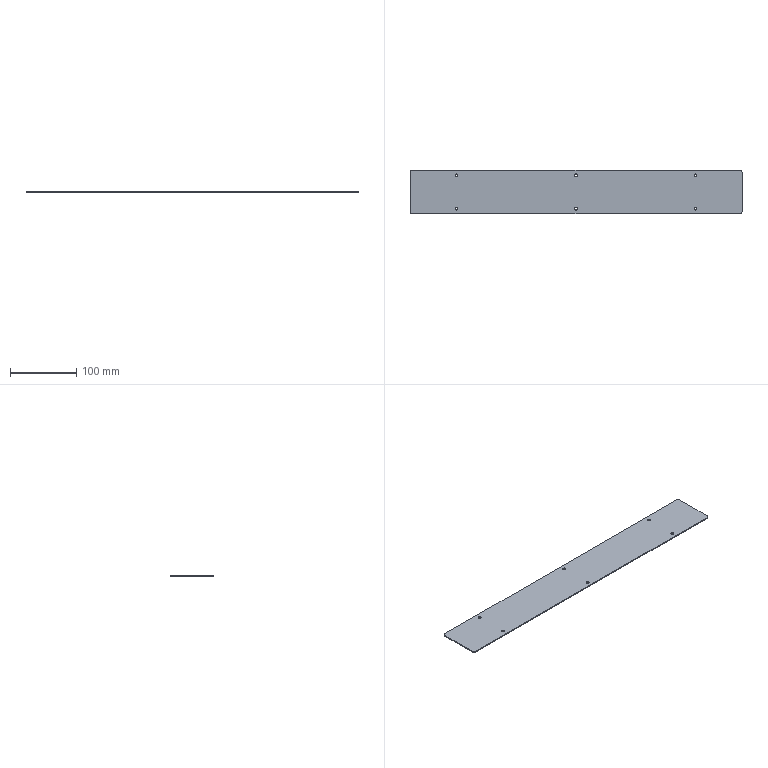Part | SolidWorks | features Fillet 1, FlatPattern 1, ICE 1, LPattern 1, SMBaseFlange 1, SheetMetal 1 | 1 solid | 22 faces | box 500 x 65 x 1.5 mm | volume 48608 mm3 | cylinder 16 | plane 6 | commonest cylinder face diameters 4.3 x12 6 x4
STEP:
#1=CARTESIAN_POINT('',(2.15,25.,-1.5));
#2=VERTEX_POINT('',#1);
#3=CARTESIAN_POINT('',(-2.15,25.,-1.5));
#4=VERTEX_POINT('',#3);
#5=CARTESIAN_POINT('',(0.,25.,-1.5));
#6=DIRECTION('',(0.,0.,-1.));
#7=DIRECTION('',(-1.,0.,0.));
#8=AXIS2_PLACEMENT_3D('',#5,#6,#7);
#9=CIRCLE('',#8,2.15);
#10=EDGE_CURVE('',#2,#4,#9,.T.);
#11=ORIENTED_EDGE('',*,*,#10,.T.);
#12=CARTESIAN_POINT('',(-2.15,25.,0.));
#13=VERTEX_POINT('',#12);
#14=CARTESIAN_POINT('',(-2.15,25.,-10.));
#15=DIRECTION('',(0.,0.,1.));
#16=VECTOR('',#15,1000.);
#17=LINE('',#14,#16);
#18=EDGE_CURVE('',#4,#13,#17,.T.);
#19=ORIENTED_EDGE('',*,*,#18,.T.);
#20=CARTESIAN_POINT('',(2.15,25.,0.));
#21=VERTEX_POINT('',#20);
#22=CARTESIAN_POINT('',(0.,25.,0.));
#23=DIRECTION('',(0.,0.,1.));
#24=DIRECTION('',(1.,0.,0.));
#25=AXIS2_PLACEMENT_3D('',#22,#23,#24);
#26=CIRCLE('',#25,2.15);
#27=EDGE_CURVE('',#13,#21,#26,.T.);
#28=ORIENTED_EDGE('',*,*,#27,.T.);
#29=CARTESIAN_POINT('',(2.15,25.,-10.));
#30=DIRECTION('',(0.,0.,1.));
#31=VECTOR('',#30,1000.);
#32=LINE('',#29,#31);
#33=EDGE_CURVE('',#2,#21,#32,.T.);
#34=ORIENTED_EDGE('',*,*,#33,.F.);
#35=EDGE_LOOP('',(#11,#19,#28,#34));
#36=FACE_OUTER_BOUND('',#35,.T.);
#37=CARTESIAN_POINT('',(0.,25.,-10.));
#38=DIRECTION('',(0.,0.,1.));
#39=DIRECTION('',(1.,0.,0.));
#40=AXIS2_PLACEMENT_3D('',#37,#38,#39);
#41=CYLINDRICAL_SURFACE('',#40,2.15);
#42=ADVANCED_FACE('',(#36),#41,.F.);
#43=CARTESIAN_POINT('',(-177.85,25.,-1.5));
#44=VERTEX_POINT('',#43);
#45=CARTESIAN_POINT('',(-182.15,25.,-1.5));
#46=VERTEX_POINT('',#45);
#47=CARTESIAN_POINT('',(-180.,25.,-1.5));
#48=DIRECTION('',(0.,0.,-1.));
#49=DIRECTION('',(-1.,0.,0.));
#50=AXIS2_PLACEMENT_3D('',#47,#48,#49);
#51=CIRCLE('',#50,2.15);
#52=EDGE_CURVE('',#44,#46,#51,.T.);
#53=ORIENTED_EDGE('',*,*,#52,.T.);
#54=CARTESIAN_POINT('',(-182.15,25.,0.));
#55=VERTEX_POINT('',#54);
#56=CARTESIAN_POINT('',(-182.15,25.,-10.));
#57=DIRECTION('',(0.,0.,1.));
#58=VECTOR('',#57,1000.);
#59=LINE('',#56,#58);
#60=EDGE_CURVE('',#46,#55,#59,.T.);
#61=ORIENTED_EDGE('',*,*,#60,.T.);
#62=CARTESIAN_POINT('',(-177.85,25.,0.));
#63=VERTEX_POINT('',#62);
#64=CARTESIAN_POINT('',(-180.,25.,0.));
#65=DIRECTION('',(0.,0.,1.));
#66=DIRECTION('',(1.,0.,0.));
#67=AXIS2_PLACEMENT_3D('',#64,#65,#66);
#68=CIRCLE('',#67,2.15);
#69=EDGE_CURVE('',#55,#63,#68,.T.);
#70=ORIENTED_EDGE('',*,*,#69,.T.);
#71=CARTESIAN_POINT('',(-177.85,25.,-10.));
#72=DIRECTION('',(0.,0.,1.));
#73=VECTOR('',#72,1000.);
#74=LINE('',#71,#73);
#75=EDGE_CURVE('',#44,#63,#74,.T.);
#76=ORIENTED_EDGE('',*,*,#75,.F.);
#77=EDGE_LOOP('',(#53,#61,#70,#76));
#78=FACE_OUTER_BOUND('',#77,.T.);
#79=CARTESIAN_POINT('',(-180.,25.,-10.));
#80=DIRECTION('',(0.,0.,1.));
#81=DIRECTION('',(1.,0.,0.));
#82=AXIS2_PLACEMENT_3D('',#79,#80,#81);
#83=CYLINDRICAL_SURFACE('',#82,2.15);
#84=ADVANCED_FACE('',(#78),#83,.F.);
#85=CARTESIAN_POINT('',(182.15,25.,-1.5));
#86=VERTEX_POINT('',#85);
#87=CARTESIAN_POINT('',(177.85,25.,-1.5));
#88=VERTEX_POINT('',#87);
#89=CARTESIAN_POINT('',(180.,25.,-1.5));
#90=DIRECTION('',(0.,0.,-1.));
#91=DIRECTION('',(-1.,0.,0.));
#92=AXIS2_PLACEMENT_3D('',#89,#90,#91);
#93=CIRCLE('',#92,2.15);
#94=EDGE_CURVE('',#86,#88,#93,.T.);
#95=ORIENTED_EDGE('',*,*,#94,.T.);
#96=CARTESIAN_POINT('',(177.85,25.,0.));
#97=VERTEX_POINT('',#96);
#98=CARTESIAN_POINT('',(177.85,25.,-10.));
#99=DIRECTION('',(0.,0.,1.));
#100=VECTOR('',#99,1000.);
#101=LINE('',#98,#100);
#102=EDGE_CURVE('',#88,#97,#101,.T.);
#103=ORIENTED_EDGE('',*,*,#102,.T.);
#104=CARTESIAN_POINT('',(182.15,25.,0.));
#105=VERTEX_POINT('',#104);
#106=CARTESIAN_POINT('',(180.,25.,0.));
#107=DIRECTION('',(0.,0.,1.));
#108=DIRECTION('',(1.,0.,0.));
#109=AXIS2_PLACEMENT_3D('',#106,#107,#108);
#110=CIRCLE('',#109,2.15);
#111=EDGE_CURVE('',#97,#105,#110,.T.);
#112=ORIENTED_EDGE('',*,*,#111,.T.);
#113=CARTESIAN_POINT('',(182.15,25.,-10.));
#114=DIRECTION('',(0.,0.,1.));
#115=VECTOR('',#114,1000.);
#116=LINE('',#113,#115);
#117=EDGE_CURVE('',#86,#105,#116,.T.);
#118=ORIENTED_EDGE('',*,*,#117,.F.);
#119=EDGE_LOOP('',(#95,#103,#112,#118));
#120=FACE_OUTER_BOUND('',#119,.T.);
#121=CARTESIAN_POINT('',(180.,25.,-10.));
#122=DIRECTION('',(0.,0.,1.));
#123=DIRECTION('',(1.,0.,0.));
#124=AXIS2_PLACEMENT_3D('',#121,#122,#123);
#125=CYLINDRICAL_SURFACE('',#124,2.15);
#126=ADVANCED_FACE('',(#120),#125,.F.);
#127=CARTESIAN_POINT('',(-177.85,-25.,-1.5));
#128=VERTEX_POINT('',#127);
#129=CARTESIAN_POINT('',(-182.15,-25.,-1.5));
#130=VERTEX_POINT('',#129);
#131=CARTESIAN_POINT('',(-180.,-25.,-1.5));
#132=DIRECTION('',(0.,0.,-1.));
#133=DIRECTION('',(-1.,0.,0.));
#134=AXIS2_PLACEMENT_3D('',#131,#132,#133);
#135=CIRCLE('',#134,2.15);
#136=EDGE_CURVE('',#128,#130,#135,.T.);
#137=ORIENTED_EDGE('',*,*,#136,.T.);
#138=CARTESIAN_POINT('',(-182.15,-25.,0.));
#139=VERTEX_POINT('',#138);
#140=CARTESIAN_POINT('',(-182.15,-25.,-10.));
#141=DIRECTION('',(0.,0.,1.));
#142=VECTOR('',#141,1000.);
#143=LINE('',#140,#142);
#144=EDGE_CURVE('',#130,#139,#143,.T.);
#145=ORIENTED_EDGE('',*,*,#144,.T.);
#146=CARTESIAN_POINT('',(-177.85,-25.,0.));
#147=VERTEX_POINT('',#146);
#148=CARTESIAN_POINT('',(-180.,-25.,0.));
#149=DIRECTION('',(0.,0.,1.));
#150=DIRECTION('',(1.,0.,0.));
#151=AXIS2_PLACEMENT_3D('',#148,#149,#150);
#152=CIRCLE('',#151,2.15);
#153=EDGE_CURVE('',#139,#147,#152,.T.);
#154=ORIENTED_EDGE('',*,*,#153,.T.);
#155=CARTESIAN_POINT('',(-177.85,-25.,-10.));
#156=DIRECTION('',(0.,0.,1.));
#157=VECTOR('',#156,1000.);
#158=LINE('',#155,#157);
#159=EDGE_CURVE('',#128,#147,#158,.T.);
#160=ORIENTED_EDGE('',*,*,#159,.F.);
#161=EDGE_LOOP('',(#137,#145,#154,#160));
#162=FACE_OUTER_BOUND('',#161,.T.);
#163=CARTESIAN_POINT('',(-180.,-25.,-10.));
#164=DIRECTION('',(0.,0.,1.));
#165=DIRECTION('',(1.,0.,0.));
#166=AXIS2_PLACEMENT_3D('',#163,#164,#165);
#167=CYLINDRICAL_SURFACE('',#166,2.15);
#168=ADVANCED_FACE('',(#162),#167,.F.);
#169=CARTESIAN_POINT('',(2.15,-25.,-1.5));
#170=VERTEX_POINT('',#169);
#171=CARTESIAN_POINT('',(-2.15,-25.,-1.5));
#172=VERTEX_POINT('',#171);
#173=CARTESIAN_POINT('',(0.,-25.,-1.5));
#174=DIRECTION('',(0.,0.,-1.));
#175=DIRECTION('',(-1.,0.,0.));
#176=AXIS2_PLACEMENT_3D('',#173,#174,#175);
#177=CIRCLE('',#176,2.15);
#178=EDGE_CURVE('',#170,#172,#177,.T.);
#179=ORIENTED_EDGE('',*,*,#178,.T.);
#180=CARTESIAN_POINT('',(-2.15,-25.,0.));
#181=VERTEX_POINT('',#180);
#182=CARTESIAN_POINT('',(-2.15,-25.,-10.));
#183=DIRECTION('',(0.,0.,1.));
#184=VECTOR('',#183,1000.);
#185=LINE('',#182,#184);
#186=EDGE_CURVE('',#172,#181,#185,.T.);
#187=ORIENTED_EDGE('',*,*,#186,.T.);
#188=CARTESIAN_POINT('',(2.15,-25.,0.));
#189=VERTEX_POINT('',#188);
#190=CARTESIAN_POINT('',(0.,-25.,0.));
#191=DIRECTION('',(0.,0.,1.));
#192=DIRECTION('',(1.,0.,0.));
#193=AXIS2_PLACEMENT_3D('',#190,#191,#192);
#194=CIRCLE('',#193,2.15);
#195=EDGE_CURVE('',#181,#189,#194,.T.);
#196=ORIENTED_EDGE('',*,*,#195,.T.);
#197=CARTESIAN_POINT('',(2.15,-25.,-10.));
#198=DIRECTION('',(0.,0.,1.));
#199=VECTOR('',#198,1000.);
#200=LINE('',#197,#199);
#201=EDGE_CURVE('',#170,#189,#200,.T.);
#202=ORIENTED_EDGE('',*,*,#201,.F.);
#203=EDGE_LOOP('',(#179,#187,#196,#202));
#204=FACE_OUTER_BOUND('',#203,.T.);
#205=CARTESIAN_POINT('',(0.,-25.,-10.));
#206=DIRECTION('',(0.,0.,1.));
#207=DIRECTION('',(1.,0.,0.));
#208=AXIS2_PLACEMENT_3D('',#205,#206,#207);
#209=CYLINDRICAL_SURFACE('',#208,2.15);
#210=ADVANCED_FACE('',(#204),#209,.F.);
#211=CARTESIAN_POINT('',(182.15,-25.,-1.5));
#212=VERTEX_POINT('',#211);
#213=CARTESIAN_POINT('',(177.85,-25.,-1.5));
#214=VERTEX_POINT('',#213);
#215=CARTESIAN_POINT('',(180.,-25.,-1.5));
#216=DIRECTION('',(0.,0.,-1.));
#217=DIRECTION('',(-1.,0.,0.));
#218=AXIS2_PLACEMENT_3D('',#215,#216,#217);
#219=CIRCLE('',#218,2.15);
#220=EDGE_CURVE('',#212,#214,#219,.T.);
#221=ORIENTED_EDGE('',*,*,#220,.T.);
#222=CARTESIAN_POINT('',(177.85,-25.,0.));
#223=VERTEX_POINT('',#222);
#224=CARTESIAN_POINT('',(177.85,-25.,-10.));
#225=DIRECTION('',(0.,0.,1.));
#226=VECTOR('',#225,1000.);
#227=LINE('',#224,#226);
#228=EDGE_CURVE('',#214,#223,#227,.T.);
#229=ORIENTED_EDGE('',*,*,#228,.T.);
#230=CARTESIAN_POINT('',(182.15,-25.,0.));
#231=VERTEX_POINT('',#230);
#232=CARTESIAN_POINT('',(180.,-25.,0.));
#233=DIRECTION('',(0.,0.,1.));
#234=DIRECTION('',(1.,0.,0.));
#235=AXIS2_PLACEMENT_3D('',#232,#233,#234);
#236=CIRCLE('',#235,2.15);
#237=EDGE_CURVE('',#223,#231,#236,.T.);
#238=ORIENTED_EDGE('',*,*,#237,.T.);
#239=CARTESIAN_POINT('',(182.15,-25.,-10.));
#240=DIRECTION('',(0.,0.,1.));
#241=VECTOR('',#240,1000.);
#242=LINE('',#239,#241);
#243=EDGE_CURVE('',#212,#231,#242,.T.);
#244=ORIENTED_EDGE('',*,*,#243,.F.);
#245=EDGE_LOOP('',(#221,#229,#238,#244));
#246=FACE_OUTER_BOUND('',#245,.T.);
#247=CARTESIAN_POINT('',(180.,-25.,-10.));
#248=DIRECTION('',(0.,0.,1.));
#249=DIRECTION('',(1.,0.,0.));
#250=AXIS2_PLACEMENT_3D('',#247,#248,#249);
#251=CYLINDRICAL_SURFACE('',#250,2.15);
#252=ADVANCED_FACE('',(#246),#251,.F.);
#253=ORIENTED_EDGE('',*,*,#228,.F.);
#254=CARTESIAN_POINT('',(180.,-25.,-1.5));
#255=DIRECTION('',(0.,0.,-1.));
#256=DIRECTION('',(-1.,0.,0.));
#257=AXIS2_PLACEMENT_3D('',#254,#255,#256);
#258=CIRCLE('',#257,2.15);
#259=EDGE_CURVE('',#214,#212,#258,.T.);
#260=ORIENTED_EDGE('',*,*,#259,.T.);
#261=ORIENTED_EDGE('',*,*,#243,.T.);
#262=CARTESIAN_POINT('',(180.,-25.,0.));
#263=DIRECTION('',(0.,0.,1.));
#264=DIRECTION('',(1.,0.,0.));
#265=AXIS2_PLACEMENT_3D('',#262,#263,#264);
#266=CIRCLE('',#265,2.15);
#267=EDGE_CURVE('',#231,#223,#266,.T.);
#268=ORIENTED_EDGE('',*,*,#267,.T.);
#269=EDGE_LOOP('',(#253,#260,#261,#268));
#270=FACE_OUTER_BOUND('',#269,.T.);
#271=CARTESIAN_POINT('',(180.,-25.,-10.));
#272=DIRECTION('',(0.,0.,1.));
#273=DIRECTION('',(1.,0.,0.));
#274=AXIS2_PLACEMENT_3D('',#271,#272,#273);
#275=CYLINDRICAL_SURFACE('',#274,2.15);
#276=ADVANCED_FACE('',(#270),#275,.F.);
#277=ORIENTED_EDGE('',*,*,#186,.F.);
#278=CARTESIAN_POINT('',(0.,-25.,-1.5));
#279=DIRECTION('',(0.,0.,-1.));
#280=DIRECTION('',(-1.,0.,0.));
#281=AXIS2_PLACEMENT_3D('',#278,#279,#280);
#282=CIRCLE('',#281,2.15);
#283=EDGE_CURVE('',#172,#170,#282,.T.);
#284=ORIENTED_EDGE('',*,*,#283,.T.);
#285=ORIENTED_EDGE('',*,*,#201,.T.);
#286=CARTESIAN_POINT('',(0.,-25.,0.));
#287=DIRECTION('',(0.,0.,1.));
#288=DIRECTION('',(1.,0.,0.));
#289=AXIS2_PLACEMENT_3D('',#286,#287,#288);
#290=CIRCLE('',#289,2.15);
#291=EDGE_CURVE('',#189,#181,#290,.T.);
#292=ORIENTED_EDGE('',*,*,#291,.T.);
#293=EDGE_LOOP('',(#277,#284,#285,#292));
#294=FACE_OUTER_BOUND('',#293,.T.);
#295=CARTESIAN_POINT('',(0.,-25.,-10.));
#296=DIRECTION('',(0.,0.,1.));
#297=DIRECTION('',(1.,0.,0.));
#298=AXIS2_PLACEMENT_3D('',#295,#296,#297);
#299=CYLINDRICAL_SURFACE('',#298,2.15);
#300=ADVANCED_FACE('',(#294),#299,.F.);
#301=ORIENTED_EDGE('',*,*,#144,.F.);
#302=CARTESIAN_POINT('',(-180.,-25.,-1.5));
#303=DIRECTION('',(0.,0.,-1.));
#304=DIRECTION('',(-1.,0.,0.));
#305=AXIS2_PLACEMENT_3D('',#302,#303,#304);
#306=CIRCLE('',#305,2.15);
#307=EDGE_CURVE('',#130,#128,#306,.T.);
#308=ORIENTED_EDGE('',*,*,#307,.T.);
#309=ORIENTED_EDGE('',*,*,#159,.T.);
#310=CARTESIAN_POINT('',(-180.,-25.,0.));
#311=DIRECTION('',(0.,0.,1.));
#312=DIRECTION('',(1.,0.,0.));
#313=AXIS2_PLACEMENT_3D('',#310,#311,#312);
#314=CIRCLE('',#313,2.15);
#315=EDGE_CURVE('',#147,#139,#314,.T.);
#316=ORIENTED_EDGE('',*,*,#315,.T.);
#317=EDGE_LOOP('',(#301,#308,#309,#316));
#318=FACE_OUTER_BOUND('',#317,.T.);
#319=CARTESIAN_POINT('',(-180.,-25.,-10.));
#320=DIRECTION('',(0.,0.,1.));
#321=DIRECTION('',(1.,0.,0.));
#322=AXIS2_PLACEMENT_3D('',#319,#320,#321);
#323=CYLINDRICAL_SURFACE('',#322,2.15);
#324=ADVANCED_FACE('',(#318),#323,.F.);
#325=ORIENTED_EDGE('',*,*,#102,.F.);
#326=CARTESIAN_POINT('',(180.,25.,-1.5));
#327=DIRECTION('',(0.,0.,-1.));
#328=DIRECTION('',(-1.,0.,0.));
#329=AXIS2_PLACEMENT_3D('',#326,#327,#328);
#330=CIRCLE('',#329,2.15);
#331=EDGE_CURVE('',#88,#86,#330,.T.);
#332=ORIENTED_EDGE('',*,*,#331,.T.);
#333=ORIENTED_EDGE('',*,*,#117,.T.);
#334=CARTESIAN_POINT('',(180.,25.,0.));
#335=DIRECTION('',(0.,0.,1.));
#336=DIRECTION('',(1.,0.,0.));
#337=AXIS2_PLACEMENT_3D('',#334,#335,#336);
#338=CIRCLE('',#337,2.15);
#339=EDGE_CURVE('',#105,#97,#338,.T.);
#340=ORIENTED_EDGE('',*,*,#339,.T.);
#341=EDGE_LOOP('',(#325,#332,#333,#340));
#342=FACE_OUTER_BOUND('',#341,.T.);
#343=CARTESIAN_POINT('',(180.,25.,-10.));
#344=DIRECTION('',(0.,0.,1.));
#345=DIRECTION('',(1.,0.,0.));
#346=AXIS2_PLACEMENT_3D('',#343,#344,#345);
#347=CYLINDRICAL_SURFACE('',#346,2.15);
#348=ADVANCED_FACE('',(#342),#347,.F.);
#349=CARTESIAN_POINT('',(250.,-29.5,-1.5));
#350=VERTEX_POINT('',#349);
#351=CARTESIAN_POINT('',(250.,29.5,-1.5));
#352=VERTEX_POINT('',#351);
#353=CARTESIAN_POINT('',(250.,-32.5,-1.5));
#354=DIRECTION('',(0.,1.,0.));
#355=VECTOR('',#354,1000.);
#356=LINE('',#353,#355);
#357=EDGE_CURVE('',#350,#352,#356,.T.);
#358=ORIENTED_EDGE('',*,*,#357,.T.);
#359=CARTESIAN_POINT('',(250.,29.5,0.));
#360=VERTEX_POINT('',#359);
#361=CARTESIAN_POINT('',(250.,29.5,-1.5));
#362=DIRECTION('',(0.,0.,1.));
#363=VECTOR('',#362,1000.);
#364=LINE('',#361,#363);
#365=EDGE_CURVE('',#352,#360,#364,.T.);
#366=ORIENTED_EDGE('',*,*,#365,.T.);
#367=CARTESIAN_POINT('',(250.,-29.5,0.));
#368=VERTEX_POINT('',#367);
#369=CARTESIAN_POINT('',(250.,-32.5,0.));
#370=DIRECTION('',(0.,1.,0.));
#371=VECTOR('',#370,1000.);
#372=LINE('',#369,#371);
#373=EDGE_CURVE('',#368,#360,#372,.T.);
#374=ORIENTED_EDGE('',*,*,#373,.F.);
#375=CARTESIAN_POINT('',(250.,-29.5,-1.5));
#376=DIRECTION('',(0.,0.,-1.));
#377=VECTOR('',#376,1000.);
#378=LINE('',#375,#377);
#379=EDGE_CURVE('',#368,#350,#378,.T.);
#380=ORIENTED_EDGE('',*,*,#379,.T.);
#381=EDGE_LOOP('',(#358,#366,#374,#380));
#382=FACE_OUTER_BOUND('',#381,.T.);
#383=CARTESIAN_POINT('',(250.,-32.5,-1.5));
#384=DIRECTION('',(1.,0.,0.));
#385=DIRECTION('',(0.,0.,-1.));
#386=AXIS2_PLACEMENT_3D('',#383,#384,#385);
#387=PLANE('',#386);
#388=ADVANCED_FACE('',(#382),#387,.T.);
#389=CARTESIAN_POINT('',(-247.,-32.5,0.));
#390=VERTEX_POINT('',#389);
#391=CARTESIAN_POINT('',(247.,-32.5,0.));
#392=VERTEX_POINT('',#391);
#393=CARTESIAN_POINT('',(-250.,-32.5,0.));
#394=DIRECTION('',(1.,0.,0.));
#395=VECTOR('',#394,1000.);
#396=LINE('',#393,#395);
#397=EDGE_CURVE('',#390,#392,#396,.T.);
#398=ORIENTED_EDGE('',*,*,#397,.F.);
#399=CARTESIAN_POINT('',(-247.,-32.5,-1.5));
#400=VERTEX_POINT('',#399);
#401=CARTESIAN_POINT('',(-247.,-32.5,-1.5));
#402=DIRECTION('',(0.,0.,-1.));
#403=VECTOR('',#402,1000.);
#404=LINE('',#401,#403);
#405=EDGE_CURVE('',#390,#400,#404,.T.);
#406=ORIENTED_EDGE('',*,*,#405,.T.);
#407=CARTESIAN_POINT('',(247.,-32.5,-1.5));
#408=VERTEX_POINT('',#407);
#409=CARTESIAN_POINT('',(-250.,-32.5,-1.5));
#410=DIRECTION('',(1.,0.,0.));
#411=VECTOR('',#410,1000.);
#412=LINE('',#409,#411);
#413=EDGE_CURVE('',#400,#408,#412,.T.);
#414=ORIENTED_EDGE('',*,*,#413,.T.);
#415=CARTESIAN_POINT('',(247.,-32.5,-1.5));
#416=DIRECTION('',(0.,0.,1.));
#417=VECTOR('',#416,1000.);
#418=LINE('',#415,#417);
#419=EDGE_CURVE('',#408,#392,#418,.T.);
#420=ORIENTED_EDGE('',*,*,#419,.T.);
#421=EDGE_LOOP('',(#398,#406,#414,#420));
#422=FACE_OUTER_BOUND('',#421,.T.);
#423=CARTESIAN_POINT('',(-250.,-32.5,-1.5));
#424=DIRECTION('',(0.,-1.,0.));
#425=DIRECTION('',(0.,0.,-1.));
#426=AXIS2_PLACEMENT_3D('',#423,#424,#425);
#427=PLANE('',#426);
#428=ADVANCED_FACE('',(#422),#427,.T.);
#429=CARTESIAN_POINT('',(-250.,29.5,-1.5));
#430=VERTEX_POINT('',#429);
#431=CARTESIAN_POINT('',(-250.,-29.5,-1.5));
#432=VERTEX_POINT('',#431);
#433=CARTESIAN_POINT('',(-250.,-32.5,-1.5));
#434=DIRECTION('',(0.,-1.,0.));
#435=VECTOR('',#434,1000.);
#436=LINE('',#433,#435);
#437=EDGE_CURVE('',#430,#432,#436,.T.);
#438=ORIENTED_EDGE('',*,*,#437,.T.);
#439=CARTESIAN_POINT('',(-250.,-29.5,0.));
#440=VERTEX_POINT('',#439);
#441=CARTESIAN_POINT('',(-250.,-29.5,-1.5));
#442=DIRECTION('',(0.,0.,1.));
#443=VECTOR('',#442,1000.);
#444=LINE('',#441,#443);
#445=EDGE_CURVE('',#432,#440,#444,.T.);
#446=ORIENTED_EDGE('',*,*,#445,.T.);
#447=CARTESIAN_POINT('',(-250.,29.5,0.));
#448=VERTEX_POINT('',#447);
#449=CARTESIAN_POINT('',(-250.,-32.5,0.));
#450=DIRECTION('',(0.,-1.,0.));
#451=VECTOR('',#450,1000.);
#452=LINE('',#449,#451);
#453=EDGE_CURVE('',#448,#440,#452,.T.);
#454=ORIENTED_EDGE('',*,*,#453,.F.);
#455=CARTESIAN_POINT('',(-250.,29.5,-1.5));
#456=DIRECTION('',(0.,0.,-1.));
#457=VECTOR('',#456,1000.);
#458=LINE('',#455,#457);
#459=EDGE_CURVE('',#448,#430,#458,.T.);
#460=ORIENTED_EDGE('',*,*,#459,.T.);
#461=EDGE_LOOP('',(#438,#446,#454,#460));
#462=FACE_OUTER_BOUND('',#461,.T.);
#463=CARTESIAN_POINT('',(-250.,-32.5,-1.5));
#464=DIRECTION('',(-1.,0.,0.));
#465=DIRECTION('',(0.,0.,1.));
#466=AXIS2_PLACEMENT_3D('',#463,#464,#465);
#467=PLANE('',#466);
#468=ADVANCED_FACE('',(#462),#467,.T.);
#469=CARTESIAN_POINT('',(247.,32.5,0.));
#470=VERTEX_POINT('',#469);
#471=CARTESIAN_POINT('',(-247.,32.5,0.));
#472=VERTEX_POINT('',#471);
#473=CARTESIAN_POINT('',(-250.,32.5,0.));
#474=DIRECTION('',(-1.,0.,0.));
#475=VECTOR('',#474,1000.);
#476=LINE('',#473,#475);
#477=EDGE_CURVE('',#470,#472,#476,.T.);
#478=ORIENTED_EDGE('',*,*,#477,.F.);
#479=CARTESIAN_POINT('',(247.,32.5,-1.5));
#480=VERTEX_POINT('',#479);
#481=CARTESIAN_POINT('',(247.,32.5,-1.5));
#482=DIRECTION('',(0.,0.,-1.));
#483=VECTOR('',#482,1000.);
#484=LINE('',#481,#483);
#485=EDGE_CURVE('',#470,#480,#484,.T.);
#486=ORIENTED_EDGE('',*,*,#485,.T.);
#487=CARTESIAN_POINT('',(-247.,32.5,-1.5));
#488=VERTEX_POINT('',#487);
#489=CARTESIAN_POINT('',(-250.,32.5,-1.5));
#490=DIRECTION('',(-1.,0.,0.));
#491=VECTOR('',#490,1000.);
#492=LINE('',#489,#491);
#493=EDGE_CURVE('',#480,#488,#492,.T.);
#494=ORIENTED_EDGE('',*,*,#493,.T.);
#495=CARTESIAN_POINT('',(-247.,32.5,-1.5));
#496=DIRECTION('',(0.,0.,1.));
#497=VECTOR('',#496,1000.);
#498=LINE('',#495,#497);
#499=EDGE_CURVE('',#488,#472,#498,.T.);
#500=ORIENTED_EDGE('',*,*,#499,.T.);
#501=EDGE_LOOP('',(#478,#486,#494,#500));
#502=FACE_OUTER_BOUND('',#501,.T.);
#503=CARTESIAN_POINT('',(-250.,32.5,-1.5));
#504=DIRECTION('',(0.,1.,0.));
#505=DIRECTION('',(0.,0.,1.));
#506=AXIS2_PLACEMENT_3D('',#503,#504,#505);
#507=PLANE('',#506);
#508=ADVANCED_FACE('',(#502),#507,.T.);
#509=ORIENTED_EDGE('',*,*,#10,.F.);
#510=CARTESIAN_POINT('',(0.,25.,-1.5));
#511=DIRECTION('',(0.,0.,-1.));
#512=DIRECTION('',(-1.,0.,0.));
#513=AXIS2_PLACEMENT_3D('',#510,#511,#512);
#514=CIRCLE('',#513,2.15);
#515=EDGE_CURVE('',#4,#2,#514,.T.);
#516=ORIENTED_EDGE('',*,*,#515,.F.);
#517=EDGE_LOOP('',(#509,#516));
#518=FACE_BOUND('',#517,.T.);
#519=ORIENTED_EDGE('',*,*,#52,.F.);
#520=CARTESIAN_POINT('',(-180.,25.,-1.5));
#521=DIRECTION('',(0.,0.,-1.));
#522=DIRECTION('',(-1.,0.,0.));
#523=AXIS2_PLACEMENT_3D('',#520,#521,#522);
#524=CIRCLE('',#523,2.15);
#525=EDGE_CURVE('',#46,#44,#524,.T.);
#526=ORIENTED_EDGE('',*,*,#525,.F.);
#527=EDGE_LOOP('',(#519,#526));
#528=FACE_BOUND('',#527,.T.);
#529=ORIENTED_EDGE('',*,*,#493,.F.);
#530=CARTESIAN_POINT('',(247.,29.5,-1.5));
#531=DIRECTION('',(0.,0.,-1.));
#532=DIRECTION('',(-1.,0.,0.));
#533=AXIS2_PLACEMENT_3D('',#530,#531,#532);
#534=CIRCLE('',#533,3.);
#535=EDGE_CURVE('',#480,#352,#534,.T.);
#536=ORIENTED_EDGE('',*,*,#535,.T.);
#537=ORIENTED_EDGE('',*,*,#357,.F.);
#538=CARTESIAN_POINT('',(247.,-29.5,-1.5));
#539=DIRECTION('',(0.,0.,-1.));
#540=DIRECTION('',(-1.,0.,0.));
#541=AXIS2_PLACEMENT_3D('',#538,#539,#540);
#542=CIRCLE('',#541,3.);
#543=EDGE_CURVE('',#350,#408,#542,.T.);
#544=ORIENTED_EDGE('',*,*,#543,.T.);
#545=ORIENTED_EDGE('',*,*,#413,.F.);
#546=CARTESIAN_POINT('',(-247.,-29.5,-1.5));
#547=DIRECTION('',(0.,0.,-1.));
#548=DIRECTION('',(-1.,0.,0.));
#549=AXIS2_PLACEMENT_3D('',#546,#547,#548);
#550=CIRCLE('',#549,3.);
#551=EDGE_CURVE('',#400,#432,#550,.T.);
#552=ORIENTED_EDGE('',*,*,#551,.T.);
#553=ORIENTED_EDGE('',*,*,#437,.F.);
#554=CARTESIAN_POINT('',(-247.,29.5,-1.5));
#555=DIRECTION('',(0.,0.,-1.));
#556=DIRECTION('',(-1.,0.,0.));
#557=AXIS2_PLACEMENT_3D('',#554,#555,#556);
#558=CIRCLE('',#557,3.);
#559=EDGE_CURVE('',#430,#488,#558,.T.);
#560=ORIENTED_EDGE('',*,*,#559,.T.);
#561=EDGE_LOOP('',(#529,#536,#537,#544,#545,#552,#553,#560));
#562=FACE_OUTER_BOUND('',#561,.T.);
#563=ORIENTED_EDGE('',*,*,#94,.F.);
#564=ORIENTED_EDGE('',*,*,#331,.F.);
#565=EDGE_LOOP('',(#563,#564));
#566=FACE_BOUND('',#565,.T.);
#567=ORIENTED_EDGE('',*,*,#136,.F.);
#568=ORIENTED_EDGE('',*,*,#307,.F.);
#569=EDGE_LOOP('',(#567,#568));
#570=FACE_BOUND('',#569,.T.);
#571=ORIENTED_EDGE('',*,*,#178,.F.);
#572=ORIENTED_EDGE('',*,*,#283,.F.);
#573=EDGE_LOOP('',(#571,#572));
#574=FACE_BOUND('',#573,.T.);
#575=ORIENTED_EDGE('',*,*,#220,.F.);
#576=ORIENTED_EDGE('',*,*,#259,.F.);
#577=EDGE_LOOP('',(#575,#576));
#578=FACE_BOUND('',#577,.T.);
#579=CARTESIAN_POINT('',(0.,0.,-1.5));
#580=DIRECTION('',(0.,0.,-1.));
#581=DIRECTION('',(-1.,0.,0.));
#582=AXIS2_PLACEMENT_3D('',#579,#580,#581);
#583=PLANE('',#582);
#584=ADVANCED_FACE('',(#518,#528,#562,#566,#570,#574,#578),#583,.T.);
#585=CARTESIAN_POINT('',(0.,25.,0.));
#586=DIRECTION('',(0.,0.,1.));
#587=DIRECTION('',(1.,0.,0.));
#588=AXIS2_PLACEMENT_3D('',#585,#586,#587);
#589=CIRCLE('',#588,2.15);
#590=EDGE_CURVE('',#21,#13,#589,.T.);
#591=ORIENTED_EDGE('',*,*,#590,.F.);
#592=ORIENTED_EDGE('',*,*,#27,.F.);
#593=EDGE_LOOP('',(#591,#592));
#594=FACE_BOUND('',#593,.T.);
#595=CARTESIAN_POINT('',(-180.,25.,0.));
#596=DIRECTION('',(0.,0.,1.));
#597=DIRECTION('',(1.,0.,0.));
#598=AXIS2_PLACEMENT_3D('',#595,#596,#597);
#599=CIRCLE('',#598,2.15);
#600=EDGE_CURVE('',#63,#55,#599,.T.);
#601=ORIENTED_EDGE('',*,*,#600,.F.);
#602=ORIENTED_EDGE('',*,*,#69,.F.);
#603=EDGE_LOOP('',(#601,#602));
#604=FACE_BOUND('',#603,.T.);
#605=ORIENTED_EDGE('',*,*,#373,.T.);
#606=CARTESIAN_POINT('',(247.,29.5,0.));
#607=DIRECTION('',(0.,0.,1.));
#608=DIRECTION('',(-1.,0.,0.));
#609=AXIS2_PLACEMENT_3D('',#606,#607,#608);
#610=CIRCLE('',#609,3.);
#611=EDGE_CURVE('',#360,#470,#610,.T.);
#612=ORIENTED_EDGE('',*,*,#611,.T.);
#613=ORIENTED_EDGE('',*,*,#477,.T.);
#614=CARTESIAN_POINT('',(-247.,29.5,0.));
#615=DIRECTION('',(0.,0.,1.));
#616=DIRECTION('',(-1.,0.,0.));
#617=AXIS2_PLACEMENT_3D('',#614,#615,#616);
#618=CIRCLE('',#617,3.);
#619=EDGE_CURVE('',#472,#448,#618,.T.);
#620=ORIENTED_EDGE('',*,*,#619,.T.);
#621=ORIENTED_EDGE('',*,*,#453,.T.);
#622=CARTESIAN_POINT('',(-247.,-29.5,0.));
#623=DIRECTION('',(0.,0.,1.));
#624=DIRECTION('',(-1.,0.,0.));
#625=AXIS2_PLACEMENT_3D('',#622,#623,#624);
#626=CIRCLE('',#625,3.);
#627=EDGE_CURVE('',#440,#390,#626,.T.);
#628=ORIENTED_EDGE('',*,*,#627,.T.);
#629=ORIENTED_EDGE('',*,*,#397,.T.);
#630=CARTESIAN_POINT('',(247.,-29.5,0.));
#631=DIRECTION('',(0.,0.,1.));
#632=DIRECTION('',(-1.,0.,0.));
#633=AXIS2_PLACEMENT_3D('',#630,#631,#632);
#634=CIRCLE('',#633,3.);
#635=EDGE_CURVE('',#392,#368,#634,.T.);
#636=ORIENTED_EDGE('',*,*,#635,.T.);
#637=EDGE_LOOP('',(#605,#612,#613,#620,#621,#628,#629,#636));
#638=FACE_OUTER_BOUND('',#637,.T.);
#639=ORIENTED_EDGE('',*,*,#339,.F.);
#640=ORIENTED_EDGE('',*,*,#111,.F.);
#641=EDGE_LOOP('',(#639,#640));
#642=FACE_BOUND('',#641,.T.);
#643=ORIENTED_EDGE('',*,*,#315,.F.);
#644=ORIENTED_EDGE('',*,*,#153,.F.);
#645=EDGE_LOOP('',(#643,#644));
#646=FACE_BOUND('',#645,.T.);
#647=ORIENTED_EDGE('',*,*,#291,.F.);
#648=ORIENTED_EDGE('',*,*,#195,.F.);
#649=EDGE_LOOP('',(#647,#648));
#650=FACE_BOUND('',#649,.T.);
#651=ORIENTED_EDGE('',*,*,#267,.F.);
#652=ORIENTED_EDGE('',*,*,#237,.F.);
#653=EDGE_LOOP('',(#651,#652));
#654=FACE_BOUND('',#653,.T.);
#655=CARTESIAN_POINT('',(0.,0.,0.));
#656=DIRECTION('',(0.,0.,-1.));
#657=DIRECTION('',(-1.,0.,0.));
#658=AXIS2_PLACEMENT_3D('',#655,#656,#657);
#659=PLANE('',#658);
#660=ADVANCED_FACE('',(#594,#604,#638,#642,#646,#650,#654),#659,.F.);
#661=ORIENTED_EDGE('',*,*,#535,.F.);
#662=ORIENTED_EDGE('',*,*,#485,.F.);
#663=ORIENTED_EDGE('',*,*,#611,.F.);
#664=ORIENTED_EDGE('',*,*,#365,.F.);
#665=EDGE_LOOP('',(#661,#662,#663,#664));
#666=FACE_OUTER_BOUND('',#665,.T.);
#667=CARTESIAN_POINT('',(247.,29.5,-1.5));
#668=DIRECTION('',(0.,0.,1.));
#669=DIRECTION('',(1.,0.,0.));
#670=AXIS2_PLACEMENT_3D('',#667,#668,#669);
#671=CYLINDRICAL_SURFACE('',#670,3.);
#672=ADVANCED_FACE('',(#666),#671,.T.);
#673=ORIENTED_EDGE('',*,*,#551,.F.);
#674=ORIENTED_EDGE('',*,*,#405,.F.);
#675=ORIENTED_EDGE('',*,*,#627,.F.);
#676=ORIENTED_EDGE('',*,*,#445,.F.);
#677=EDGE_LOOP('',(#673,#674,#675,#676));
#678=FACE_OUTER_BOUND('',#677,.T.);
#679=CARTESIAN_POINT('',(-247.,-29.5,-1.5));
#680=DIRECTION('',(0.,0.,1.));
#681=DIRECTION('',(1.,0.,0.));
#682=AXIS2_PLACEMENT_3D('',#679,#680,#681);
#683=CYLINDRICAL_SURFACE('',#682,3.);
#684=ADVANCED_FACE('',(#678),#683,.T.);
#685=ORIENTED_EDGE('',*,*,#543,.F.);
#686=ORIENTED_EDGE('',*,*,#379,.F.);
#687=ORIENTED_EDGE('',*,*,#635,.F.);
#688=ORIENTED_EDGE('',*,*,#419,.F.);
#689=EDGE_LOOP('',(#685,#686,#687,#688));
#690=FACE_OUTER_BOUND('',#689,.T.);
#691=CARTESIAN_POINT('',(247.,-29.5,-1.5));
#692=DIRECTION('',(0.,0.,1.));
#693=DIRECTION('',(1.,0.,0.));
#694=AXIS2_PLACEMENT_3D('',#691,#692,#693);
#695=CYLINDRICAL_SURFACE('',#694,3.);
#696=ADVANCED_FACE('',(#690),#695,.T.);
#697=ORIENTED_EDGE('',*,*,#559,.F.);
#698=ORIENTED_EDGE('',*,*,#459,.F.);
#699=ORIENTED_EDGE('',*,*,#619,.F.);
#700=ORIENTED_EDGE('',*,*,#499,.F.);
#701=EDGE_LOOP('',(#697,#698,#699,#700));
#702=FACE_OUTER_BOUND('',#701,.T.);
#703=CARTESIAN_POINT('',(-247.,29.5,-1.5));
#704=DIRECTION('',(0.,0.,1.));
#705=DIRECTION('',(1.,0.,0.));
#706=AXIS2_PLACEMENT_3D('',#703,#704,#705);
#707=CYLINDRICAL_SURFACE('',#706,3.);
#708=ADVANCED_FACE('',(#702),#707,.T.);
#709=ORIENTED_EDGE('',*,*,#60,.F.);
#710=ORIENTED_EDGE('',*,*,#525,.T.);
#711=ORIENTED_EDGE('',*,*,#75,.T.);
#712=ORIENTED_EDGE('',*,*,#600,.T.);
#713=EDGE_LOOP('',(#709,#710,#711,#712));
#714=FACE_OUTER_BOUND('',#713,.T.);
#715=CARTESIAN_POINT('',(-180.,25.,-10.));
#716=DIRECTION('',(0.,0.,1.));
#717=DIRECTION('',(1.,0.,0.));
#718=AXIS2_PLACEMENT_3D('',#715,#716,#717);
#719=CYLINDRICAL_SURFACE('',#718,2.15);
#720=ADVANCED_FACE('',(#714),#719,.F.);
#721=ORIENTED_EDGE('',*,*,#18,.F.);
#722=ORIENTED_EDGE('',*,*,#515,.T.);
#723=ORIENTED_EDGE('',*,*,#33,.T.);
#724=ORIENTED_EDGE('',*,*,#590,.T.);
#725=EDGE_LOOP('',(#721,#722,#723,#724));
#726=FACE_OUTER_BOUND('',#725,.T.);
#727=CARTESIAN_POINT('',(0.,25.,-10.));
#728=DIRECTION('',(0.,0.,1.));
#729=DIRECTION('',(1.,0.,0.));
#730=AXIS2_PLACEMENT_3D('',#727,#728,#729);
#731=CYLINDRICAL_SURFACE('',#730,2.15);
#732=ADVANCED_FACE('',(#726),#731,.F.);
#733=CLOSED_SHELL('',(#42,#84,#126,#168,#210,#252,#276,#300,#324,#348,#388,#428,#468,#508,#584,#660,#672,#684,#696,#708,#720,#732));
#734=MANIFOLD_SOLID_BREP('',#733);
#735=CARTESIAN_POINT('',(0.,0.,0.));
#736=DIRECTION('',(0.,0.,1.));
#737=DIRECTION('',(1.,0.,0.));
#738=AXIS2_PLACEMENT_3D('',#735,#736,#737);
#739=(LENGTH_UNIT()NAMED_UNIT(*)SI_UNIT(.MILLI.,.METRE.));
#740=UNCERTAINTY_MEASURE_WITH_UNIT(LENGTH_MEASURE(0.00001),#739,'','');
#741=(NAMED_UNIT(*)PLANE_ANGLE_UNIT()SI_UNIT($,.RADIAN.));
#742=(NAMED_UNIT(*)SI_UNIT($,.STERADIAN.)SOLID_ANGLE_UNIT());
#743=(GEOMETRIC_REPRESENTATION_CONTEXT(3)GLOBAL_UNCERTAINTY_ASSIGNED_CONTEXT((#740))GLOBAL_UNIT_ASSIGNED_CONTEXT((#739,#741,#742))REPRESENTATION_CONTEXT('',''));
#744=ADVANCED_BREP_SHAPE_REPRESENTATION('',(#734,#738),#743);